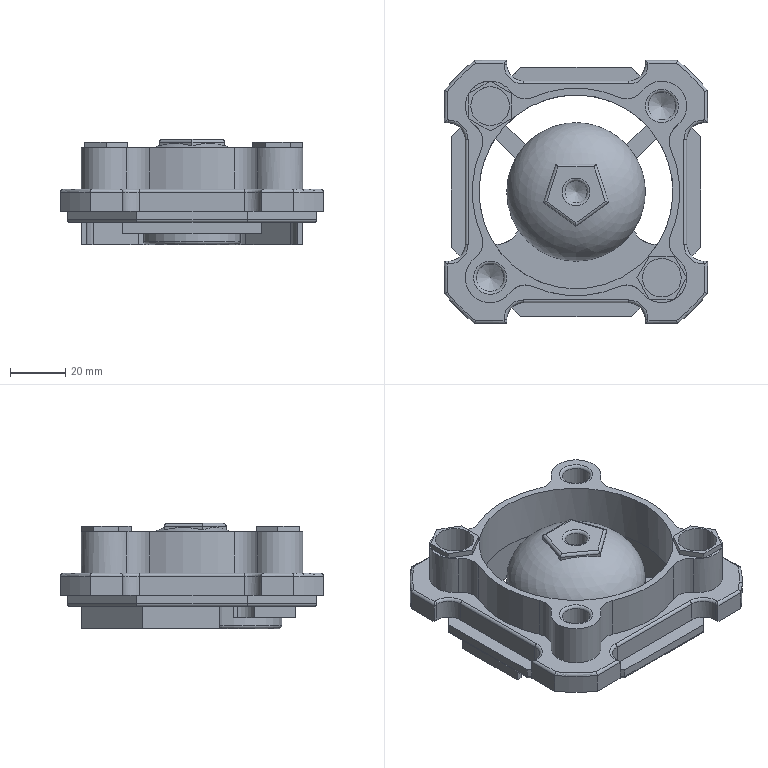Part | 1 solid | 211 faces | box 95 x 95 x 38 mm | volume 106989 mm3 | plane 101 | cylinder 89 | torus 17 | cone 3 | spline 1 | commonest cylinder face diameters 2 x33 12 x10 14 x10 8 x7 18 x6 16 x4